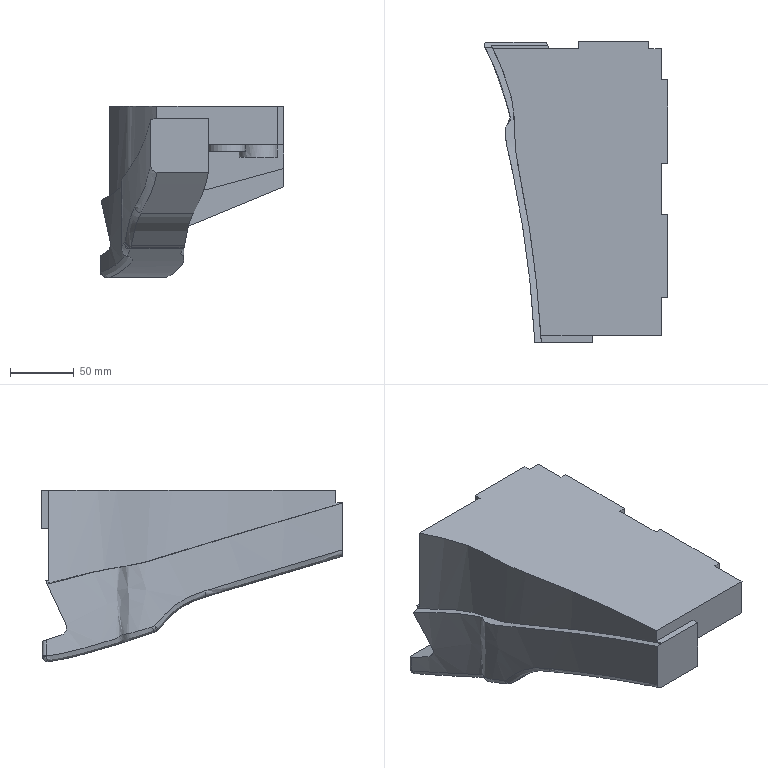Part | NX | features solid 2 | 1 solid | 64 faces | box 143.531 x 236.138 x 134.527 mm | volume 1559067 mm3 | plane 38 | spline 16 | cylinder 9 | sphere 1 | commonest cylinder face diameters 30 x5 10 x2 4 x1 12 x1